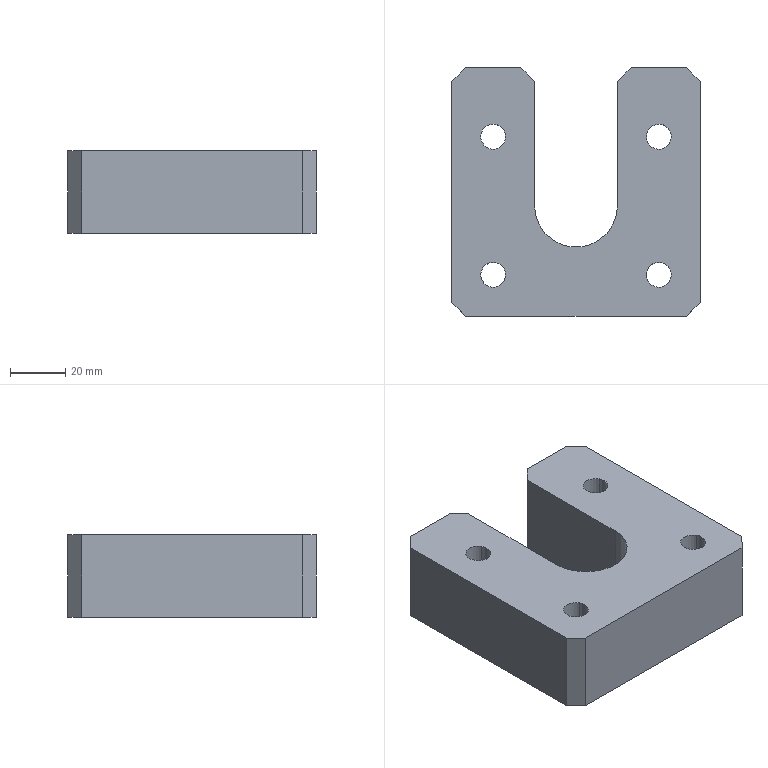Part | CATIA | 1 solid | 36 faces | box 90 x 90 x 30 mm | volume 170727 mm3 | plane 19 | cylinder 17 | commonest cylinder face diameters 9 x8 15 x8 30 x1
STEP:
#1=CARTESIAN_POINT('',(500.,-120.,-5.5));
#2=VERTEX_POINT('',#1);
#3=CARTESIAN_POINT('',(500.,-120.,24.5));
#4=VERTEX_POINT('',#3);
#5=CARTESIAN_POINT('',(500.,-120.,9.5));
#6=DIRECTION('',(0.,0.,-1.));
#7=VECTOR('',#6,1.);
#8=LINE('',#5,#7);
#9=EDGE_CURVE('',#2,#4,#8,.F.);
#10=ORIENTED_EDGE('',*,*,#9,.F.);
#11=CARTESIAN_POINT('',(495.,-125.,-5.5));
#12=VERTEX_POINT('',#11);
#13=CARTESIAN_POINT('',(497.5,-122.5,-5.5));
#14=DIRECTION('',(0.7071,0.7071,0.));
#15=VECTOR('',#14,1.);
#16=LINE('',#13,#15);
#17=EDGE_CURVE('',#2,#12,#16,.F.);
#18=ORIENTED_EDGE('',*,*,#17,.T.);
#19=CARTESIAN_POINT('',(495.,-125.,24.5));
#20=VERTEX_POINT('',#19);
#21=CARTESIAN_POINT('',(495.,-125.,9.5));
#22=DIRECTION('',(0.,0.,-1.));
#23=VECTOR('',#22,1.);
#24=LINE('',#21,#23);
#25=EDGE_CURVE('',#12,#20,#24,.F.);
#26=ORIENTED_EDGE('',*,*,#25,.T.);
#27=CARTESIAN_POINT('',(497.5,-122.5,24.5));
#28=DIRECTION('',(0.7071,0.7071,0.));
#29=VECTOR('',#28,1.);
#30=LINE('',#27,#29);
#31=EDGE_CURVE('',#20,#4,#30,.T.);
#32=ORIENTED_EDGE('',*,*,#31,.T.);
#33=EDGE_LOOP('',(#10,#18,#26,#32));
#34=FACE_OUTER_BOUND('',#33,.T.);
#35=CARTESIAN_POINT('',(495.,-125.,30.5));
#36=DIRECTION('',(0.7071,-0.7071,0.));
#37=DIRECTION('',(0.,0.,-1.));
#38=AXIS2_PLACEMENT_3D('',#35,#36,#37);
#39=PLANE('',#38);
#40=ADVANCED_FACE('',(#34),#39,.F.);
#41=CARTESIAN_POINT('',(495.,-205.,-5.5));
#42=VERTEX_POINT('',#41);
#43=CARTESIAN_POINT('',(495.,-205.,24.5));
#44=VERTEX_POINT('',#43);
#45=CARTESIAN_POINT('',(495.,-205.,9.5));
#46=DIRECTION('',(0.,0.,1.));
#47=VECTOR('',#46,1.);
#48=LINE('',#45,#47);
#49=EDGE_CURVE('',#42,#44,#48,.T.);
#50=ORIENTED_EDGE('',*,*,#49,.T.);
#51=CARTESIAN_POINT('',(495.,-165.,24.5));
#52=DIRECTION('',(0.,1.,0.));
#53=VECTOR('',#52,1.);
#54=LINE('',#51,#53);
#55=EDGE_CURVE('',#20,#44,#54,.F.);
#56=ORIENTED_EDGE('',*,*,#55,.F.);
#57=ORIENTED_EDGE('',*,*,#25,.F.);
#58=CARTESIAN_POINT('',(495.,-165.,-5.5));
#59=DIRECTION('',(0.,1.,0.));
#60=VECTOR('',#59,1.);
#61=LINE('',#58,#60);
#62=EDGE_CURVE('',#12,#42,#61,.F.);
#63=ORIENTED_EDGE('',*,*,#62,.T.);
#64=EDGE_LOOP('',(#50,#56,#57,#63));
#65=FACE_OUTER_BOUND('',#64,.T.);
#66=CARTESIAN_POINT('',(495.,-210.,-5.5));
#67=DIRECTION('',(1.,0.,0.));
#68=DIRECTION('',(0.,1.,0.));
#69=AXIS2_PLACEMENT_3D('',#66,#67,#68);
#70=PLANE('',#69);
#71=ADVANCED_FACE('',(#65),#70,.F.);
#72=ORIENTED_EDGE('',*,*,#49,.F.);
#73=CARTESIAN_POINT('',(500.,-210.,-5.5));
#74=VERTEX_POINT('',#73);
#75=CARTESIAN_POINT('',(497.5,-207.5,-5.5));
#76=DIRECTION('',(0.7071,-0.7071,0.));
#77=VECTOR('',#76,1.);
#78=LINE('',#75,#77);
#79=EDGE_CURVE('',#42,#74,#78,.T.);
#80=ORIENTED_EDGE('',*,*,#79,.T.);
#81=CARTESIAN_POINT('',(500.,-210.,24.5));
#82=VERTEX_POINT('',#81);
#83=CARTESIAN_POINT('',(500.,-210.,9.5));
#84=DIRECTION('',(0.,0.,1.));
#85=VECTOR('',#84,1.);
#86=LINE('',#83,#85);
#87=EDGE_CURVE('',#74,#82,#86,.T.);
#88=ORIENTED_EDGE('',*,*,#87,.T.);
#89=CARTESIAN_POINT('',(497.5,-207.5,24.5));
#90=DIRECTION('',(0.7071,-0.7071,0.));
#91=VECTOR('',#90,1.);
#92=LINE('',#89,#91);
#93=EDGE_CURVE('',#82,#44,#92,.F.);
#94=ORIENTED_EDGE('',*,*,#93,.T.);
#95=EDGE_LOOP('',(#72,#80,#88,#94));
#96=FACE_OUTER_BOUND('',#95,.T.);
#97=CARTESIAN_POINT('',(495.,-205.,-11.5));
#98=DIRECTION('',(0.7071,0.7071,0.));
#99=DIRECTION('',(0.,0.,1.));
#100=AXIS2_PLACEMENT_3D('',#97,#98,#99);
#101=PLANE('',#100);
#102=ADVANCED_FACE('',(#96),#101,.F.);
#103=CARTESIAN_POINT('',(580.,-210.,-5.5));
#104=VERTEX_POINT('',#103);
#105=CARTESIAN_POINT('',(580.,-210.,24.5));
#106=VERTEX_POINT('',#105);
#107=CARTESIAN_POINT('',(580.,-210.,9.5));
#108=DIRECTION('',(0.,0.,-1.));
#109=VECTOR('',#108,1.);
#110=LINE('',#107,#109);
#111=EDGE_CURVE('',#104,#106,#110,.F.);
#112=ORIENTED_EDGE('',*,*,#111,.T.);
#113=CARTESIAN_POINT('',(540.,-210.,24.5));
#114=DIRECTION('',(-1.,0.,0.));
#115=VECTOR('',#114,1.);
#116=LINE('',#113,#115);
#117=EDGE_CURVE('',#82,#106,#116,.F.);
#118=ORIENTED_EDGE('',*,*,#117,.F.);
#119=ORIENTED_EDGE('',*,*,#87,.F.);
#120=CARTESIAN_POINT('',(540.,-210.,-5.5));
#121=DIRECTION('',(-1.,0.,0.));
#122=VECTOR('',#121,1.);
#123=LINE('',#120,#122);
#124=EDGE_CURVE('',#74,#104,#123,.F.);
#125=ORIENTED_EDGE('',*,*,#124,.T.);
#126=EDGE_LOOP('',(#112,#118,#119,#125));
#127=FACE_OUTER_BOUND('',#126,.T.);
#128=CARTESIAN_POINT('',(585.,-210.,-5.5));
#129=DIRECTION('',(0.,1.,0.));
#130=DIRECTION('',(-1.,0.,0.));
#131=AXIS2_PLACEMENT_3D('',#128,#129,#130);
#132=PLANE('',#131);
#133=ADVANCED_FACE('',(#127),#132,.F.);
#134=ORIENTED_EDGE('',*,*,#111,.F.);
#135=CARTESIAN_POINT('',(585.,-205.,-5.5));
#136=VERTEX_POINT('',#135);
#137=CARTESIAN_POINT('',(582.5,-207.5,-5.5));
#138=DIRECTION('',(-0.7071,-0.7071,0.));
#139=VECTOR('',#138,1.);
#140=LINE('',#137,#139);
#141=EDGE_CURVE('',#104,#136,#140,.F.);
#142=ORIENTED_EDGE('',*,*,#141,.T.);
#143=CARTESIAN_POINT('',(585.,-205.,24.5));
#144=VERTEX_POINT('',#143);
#145=CARTESIAN_POINT('',(585.,-205.,9.5));
#146=DIRECTION('',(0.,0.,-1.));
#147=VECTOR('',#146,1.);
#148=LINE('',#145,#147);
#149=EDGE_CURVE('',#136,#144,#148,.F.);
#150=ORIENTED_EDGE('',*,*,#149,.T.);
#151=CARTESIAN_POINT('',(582.5,-207.5,24.5));
#152=DIRECTION('',(-0.7071,-0.7071,0.));
#153=VECTOR('',#152,1.);
#154=LINE('',#151,#153);
#155=EDGE_CURVE('',#144,#106,#154,.T.);
#156=ORIENTED_EDGE('',*,*,#155,.T.);
#157=EDGE_LOOP('',(#134,#142,#150,#156));
#158=FACE_OUTER_BOUND('',#157,.T.);
#159=CARTESIAN_POINT('',(585.,-205.,30.5));
#160=DIRECTION('',(-0.7071,0.7071,0.));
#161=DIRECTION('',(0.,0.,-1.));
#162=AXIS2_PLACEMENT_3D('',#159,#160,#161);
#163=PLANE('',#162);
#164=ADVANCED_FACE('',(#158),#163,.F.);
#165=CARTESIAN_POINT('',(585.,-125.,-5.5));
#166=VERTEX_POINT('',#165);
#167=CARTESIAN_POINT('',(585.,-125.,24.5));
#168=VERTEX_POINT('',#167);
#169=CARTESIAN_POINT('',(585.,-125.,9.5));
#170=DIRECTION('',(0.,0.,1.));
#171=VECTOR('',#170,1.);
#172=LINE('',#169,#171);
#173=EDGE_CURVE('',#166,#168,#172,.T.);
#174=ORIENTED_EDGE('',*,*,#173,.T.);
#175=CARTESIAN_POINT('',(585.,-165.,24.5));
#176=DIRECTION('',(0.,-1.,0.));
#177=VECTOR('',#176,1.);
#178=LINE('',#175,#177);
#179=EDGE_CURVE('',#144,#168,#178,.F.);
#180=ORIENTED_EDGE('',*,*,#179,.F.);
#181=ORIENTED_EDGE('',*,*,#149,.F.);
#182=CARTESIAN_POINT('',(585.,-165.,-5.5));
#183=DIRECTION('',(0.,-1.,0.));
#184=VECTOR('',#183,1.);
#185=LINE('',#182,#184);
#186=EDGE_CURVE('',#136,#166,#185,.F.);
#187=ORIENTED_EDGE('',*,*,#186,.T.);
#188=EDGE_LOOP('',(#174,#180,#181,#187));
#189=FACE_OUTER_BOUND('',#188,.T.);
#190=CARTESIAN_POINT('',(585.,-120.,-5.5));
#191=DIRECTION('',(-1.,0.,0.));
#192=DIRECTION('',(0.,-1.,0.));
#193=AXIS2_PLACEMENT_3D('',#190,#191,#192);
#194=PLANE('',#193);
#195=ADVANCED_FACE('',(#189),#194,.F.);
#196=ORIENTED_EDGE('',*,*,#173,.F.);
#197=CARTESIAN_POINT('',(580.,-120.,-5.5));
#198=VERTEX_POINT('',#197);
#199=CARTESIAN_POINT('',(582.5,-122.5,-5.5));
#200=DIRECTION('',(-0.7071,0.7071,0.));
#201=VECTOR('',#200,1.);
#202=LINE('',#199,#201);
#203=EDGE_CURVE('',#166,#198,#202,.T.);
#204=ORIENTED_EDGE('',*,*,#203,.T.);
#205=CARTESIAN_POINT('',(580.,-120.,24.5));
#206=VERTEX_POINT('',#205);
#207=CARTESIAN_POINT('',(580.,-120.,9.5));
#208=DIRECTION('',(0.,0.,1.));
#209=VECTOR('',#208,1.);
#210=LINE('',#207,#209);
#211=EDGE_CURVE('',#198,#206,#210,.T.);
#212=ORIENTED_EDGE('',*,*,#211,.T.);
#213=CARTESIAN_POINT('',(582.5,-122.5,24.5));
#214=DIRECTION('',(-0.7071,0.7071,0.));
#215=VECTOR('',#214,1.);
#216=LINE('',#213,#215);
#217=EDGE_CURVE('',#206,#168,#216,.F.);
#218=ORIENTED_EDGE('',*,*,#217,.T.);
#219=EDGE_LOOP('',(#196,#204,#212,#218));
#220=FACE_OUTER_BOUND('',#219,.T.);
#221=CARTESIAN_POINT('',(585.,-125.,-11.5));
#222=DIRECTION('',(-0.7071,-0.7071,0.));
#223=DIRECTION('',(0.,0.,1.));
#224=AXIS2_PLACEMENT_3D('',#221,#222,#223);
#225=PLANE('',#224);
#226=ADVANCED_FACE('',(#220),#225,.F.);
#227=CARTESIAN_POINT('',(576.582,-141.404,9.5));
#228=VERTEX_POINT('',#227);
#229=CARTESIAN_POINT('',(563.418,-148.596,9.5));
#230=VERTEX_POINT('',#229);
#231=CARTESIAN_POINT('',(570.,-145.,9.5));
#232=DIRECTION('',(0.,0.,1.));
#233=AXIS2_PLACEMENT_3D('',#231,#232,$);
#234=CIRCLE('',#233,7.5);
#235=EDGE_CURVE('',#228,#230,#234,.T.);
#236=ORIENTED_EDGE('',*,*,#235,.F.);
#237=CARTESIAN_POINT('',(570.,-145.,9.5));
#238=DIRECTION('',(0.,0.,1.));
#239=AXIS2_PLACEMENT_3D('',#237,#238,$);
#240=CIRCLE('',#239,7.5);
#241=EDGE_CURVE('',#230,#228,#240,.T.);
#242=ORIENTED_EDGE('',*,*,#241,.F.);
#243=EDGE_LOOP('',(#236,#242));
#244=FACE_OUTER_BOUND('',#243,.T.);
#245=CARTESIAN_POINT('',(566.051,-147.157,9.5));
#246=VERTEX_POINT('',#245);
#247=CARTESIAN_POINT('',(573.949,-142.843,9.5));
#248=VERTEX_POINT('',#247);
#249=CARTESIAN_POINT('',(570.,-145.,9.5));
#250=DIRECTION('',(0.,0.,1.));
#251=AXIS2_PLACEMENT_3D('',#249,#250,$);
#252=CIRCLE('',#251,4.5);
#253=EDGE_CURVE('',#246,#248,#252,.T.);
#254=ORIENTED_EDGE('',*,*,#253,.T.);
#255=CARTESIAN_POINT('',(570.,-145.,9.5));
#256=DIRECTION('',(0.,0.,1.));
#257=AXIS2_PLACEMENT_3D('',#255,#256,$);
#258=CIRCLE('',#257,4.5);
#259=EDGE_CURVE('',#248,#246,#258,.T.);
#260=ORIENTED_EDGE('',*,*,#259,.T.);
#261=EDGE_LOOP('',(#254,#260));
#262=FACE_BOUND('',#261,.T.);
#263=CARTESIAN_POINT('',(574.5,-195.,9.5));
#264=DIRECTION('',(0.,0.,1.));
#265=DIRECTION('',(1.,0.,0.));
#266=AXIS2_PLACEMENT_3D('',#263,#264,#265);
#267=PLANE('',#266);
#268=ADVANCED_FACE('',(#244,#262),#267,.F.);
#269=CARTESIAN_POINT('',(563.418,-148.596,-5.5));
#270=VERTEX_POINT('',#269);
#271=CARTESIAN_POINT('',(576.582,-141.404,-5.5));
#272=VERTEX_POINT('',#271);
#273=CARTESIAN_POINT('',(570.,-145.,-5.5));
#274=DIRECTION('',(0.,0.,1.));
#275=AXIS2_PLACEMENT_3D('',#273,#274,$);
#276=CIRCLE('',#275,7.5);
#277=EDGE_CURVE('',#270,#272,#276,.T.);
#278=ORIENTED_EDGE('',*,*,#277,.F.);
#279=CARTESIAN_POINT('',(563.418,-148.596,1.8));
#280=DIRECTION('',(0.,0.,1.));
#281=VECTOR('',#280,1.);
#282=LINE('',#279,#281);
#283=EDGE_CURVE('',#230,#270,#282,.F.);
#284=ORIENTED_EDGE('',*,*,#283,.F.);
#285=ORIENTED_EDGE('',*,*,#241,.T.);
#286=CARTESIAN_POINT('',(576.582,-141.404,1.8));
#287=DIRECTION('',(0.,0.,1.));
#288=VECTOR('',#287,1.);
#289=LINE('',#286,#288);
#290=EDGE_CURVE('',#228,#272,#289,.F.);
#291=ORIENTED_EDGE('',*,*,#290,.T.);
#292=EDGE_LOOP('',(#278,#284,#285,#291));
#293=FACE_OUTER_BOUND('',#292,.T.);
#294=CARTESIAN_POINT('',(570.,-145.,-5.4));
#295=DIRECTION('',(0.,0.,1.));
#296=DIRECTION('',(0.8776,0.4794,0.));
#297=AXIS2_PLACEMENT_3D('',#294,#295,#296);
#298=CYLINDRICAL_SURFACE('',#297,7.5);
#299=ADVANCED_FACE('',(#293),#298,.F.);
#300=CARTESIAN_POINT('',(570.,-145.,-5.5));
#301=DIRECTION('',(0.,0.,1.));
#302=AXIS2_PLACEMENT_3D('',#300,#301,$);
#303=CIRCLE('',#302,7.5);
#304=EDGE_CURVE('',#272,#270,#303,.T.);
#305=ORIENTED_EDGE('',*,*,#304,.F.);
#306=ORIENTED_EDGE('',*,*,#290,.F.);
#307=ORIENTED_EDGE('',*,*,#235,.T.);
#308=ORIENTED_EDGE('',*,*,#283,.T.);
#309=EDGE_LOOP('',(#305,#306,#307,#308));
#310=FACE_OUTER_BOUND('',#309,.T.);
#311=ADVANCED_FACE('',(#310),#298,.F.);
#312=CARTESIAN_POINT('',(573.949,-142.843,24.5));
#313=VERTEX_POINT('',#312);
#314=CARTESIAN_POINT('',(566.051,-147.157,24.5));
#315=VERTEX_POINT('',#314);
#316=CARTESIAN_POINT('',(570.,-145.,24.5));
#317=DIRECTION('',(0.,0.,1.));
#318=AXIS2_PLACEMENT_3D('',#316,#317,$);
#319=CIRCLE('',#318,4.5);
#320=EDGE_CURVE('',#313,#315,#319,.T.);
#321=ORIENTED_EDGE('',*,*,#320,.T.);
#322=CARTESIAN_POINT('',(566.051,-147.157,17.2));
#323=DIRECTION('',(0.,0.,1.));
#324=VECTOR('',#323,1.);
#325=LINE('',#322,#324);
#326=EDGE_CURVE('',#315,#246,#325,.F.);
#327=ORIENTED_EDGE('',*,*,#326,.T.);
#328=ORIENTED_EDGE('',*,*,#259,.F.);
#329=CARTESIAN_POINT('',(573.949,-142.843,17.2));
#330=DIRECTION('',(0.,0.,1.));
#331=VECTOR('',#330,1.);
#332=LINE('',#329,#331);
#333=EDGE_CURVE('',#313,#248,#332,.F.);
#334=ORIENTED_EDGE('',*,*,#333,.F.);
#335=EDGE_LOOP('',(#321,#327,#328,#334));
#336=FACE_OUTER_BOUND('',#335,.T.);
#337=CARTESIAN_POINT('',(570.,-145.,-5.4));
#338=DIRECTION('',(0.,0.,1.));
#339=DIRECTION('',(0.8776,0.4794,0.));
#340=AXIS2_PLACEMENT_3D('',#337,#338,#339);
#341=CYLINDRICAL_SURFACE('',#340,4.5);
#342=ADVANCED_FACE('',(#336),#341,.F.);
#343=CARTESIAN_POINT('',(570.,-145.,24.5));
#344=DIRECTION('',(0.,0.,1.));
#345=AXIS2_PLACEMENT_3D('',#343,#344,$);
#346=CIRCLE('',#345,4.5);
#347=EDGE_CURVE('',#315,#313,#346,.T.);
#348=ORIENTED_EDGE('',*,*,#347,.T.);
#349=ORIENTED_EDGE('',*,*,#333,.T.);
#350=ORIENTED_EDGE('',*,*,#253,.F.);
#351=ORIENTED_EDGE('',*,*,#326,.F.);
#352=EDGE_LOOP('',(#348,#349,#350,#351));
#353=FACE_OUTER_BOUND('',#352,.T.);
#354=ADVANCED_FACE('',(#353),#341,.F.);
#355=CARTESIAN_POINT('',(516.582,-191.404,9.5));
#356=VERTEX_POINT('',#355);
#357=CARTESIAN_POINT('',(503.418,-198.596,9.5));
#358=VERTEX_POINT('',#357);
#359=CARTESIAN_POINT('',(510.,-195.,9.5));
#360=DIRECTION('',(0.,0.,1.));
#361=AXIS2_PLACEMENT_3D('',#359,#360,$);
#362=CIRCLE('',#361,7.5);
#363=EDGE_CURVE('',#356,#358,#362,.T.);
#364=ORIENTED_EDGE('',*,*,#363,.F.);
#365=CARTESIAN_POINT('',(510.,-195.,9.5));
#366=DIRECTION('',(0.,0.,1.));
#367=AXIS2_PLACEMENT_3D('',#365,#366,$);
#368=CIRCLE('',#367,7.5);
#369=EDGE_CURVE('',#358,#356,#368,.T.);
#370=ORIENTED_EDGE('',*,*,#369,.F.);
#371=EDGE_LOOP('',(#364,#370));
#372=FACE_OUTER_BOUND('',#371,.T.);
#373=CARTESIAN_POINT('',(506.051,-197.157,9.5));
#374=VERTEX_POINT('',#373);
#375=CARTESIAN_POINT('',(513.949,-192.843,9.5));
#376=VERTEX_POINT('',#375);
#377=CARTESIAN_POINT('',(510.,-195.,9.5));
#378=DIRECTION('',(0.,0.,1.));
#379=AXIS2_PLACEMENT_3D('',#377,#378,$);
#380=CIRCLE('',#379,4.5);
#381=EDGE_CURVE('',#374,#376,#380,.T.);
#382=ORIENTED_EDGE('',*,*,#381,.T.);
#383=CARTESIAN_POINT('',(510.,-195.,9.5));
#384=DIRECTION('',(0.,0.,1.));
#385=AXIS2_PLACEMENT_3D('',#383,#384,$);
#386=CIRCLE('',#385,4.5);
#387=EDGE_CURVE('',#376,#374,#386,.T.);
#388=ORIENTED_EDGE('',*,*,#387,.T.);
#389=EDGE_LOOP('',(#382,#388));
#390=FACE_BOUND('',#389,.T.);
#391=ADVANCED_FACE('',(#372,#390),#267,.F.);
#392=CARTESIAN_POINT('',(503.418,-198.596,-5.5));
#393=VERTEX_POINT('',#392);
#394=CARTESIAN_POINT('',(516.582,-191.404,-5.5));
#395=VERTEX_POINT('',#394);
#396=CARTESIAN_POINT('',(510.,-195.,-5.5));
#397=DIRECTION('',(0.,0.,1.));
#398=AXIS2_PLACEMENT_3D('',#396,#397,$);
#399=CIRCLE('',#398,7.5);
#400=EDGE_CURVE('',#393,#395,#399,.T.);
#401=ORIENTED_EDGE('',*,*,#400,.F.);
#402=CARTESIAN_POINT('',(503.418,-198.596,1.8));
#403=DIRECTION('',(0.,0.,1.));
#404=VECTOR('',#403,1.);
#405=LINE('',#402,#404);
#406=EDGE_CURVE('',#358,#393,#405,.F.);
#407=ORIENTED_EDGE('',*,*,#406,.F.);
#408=ORIENTED_EDGE('',*,*,#369,.T.);
#409=CARTESIAN_POINT('',(516.582,-191.404,1.8));
#410=DIRECTION('',(0.,0.,1.));
#411=VECTOR('',#410,1.);
#412=LINE('',#409,#411);
#413=EDGE_CURVE('',#356,#395,#412,.F.);
#414=ORIENTED_EDGE('',*,*,#413,.T.);
#415=EDGE_LOOP('',(#401,#407,#408,#414));
#416=FACE_OUTER_BOUND('',#415,.T.);
#417=CARTESIAN_POINT('',(510.,-195.,-5.4));
#418=DIRECTION('',(0.,0.,1.));
#419=DIRECTION('',(0.8776,0.4794,0.));
#420=AXIS2_PLACEMENT_3D('',#417,#418,#419);
#421=CYLINDRICAL_SURFACE('',#420,7.5);
#422=ADVANCED_FACE('',(#416),#421,.F.);
#423=CARTESIAN_POINT('',(510.,-195.,-5.5));
#424=DIRECTION('',(0.,0.,1.));
#425=AXIS2_PLACEMENT_3D('',#423,#424,$);
#426=CIRCLE('',#425,7.5);
#427=EDGE_CURVE('',#395,#393,#426,.T.);
#428=ORIENTED_EDGE('',*,*,#427,.F.);
#429=ORIENTED_EDGE('',*,*,#413,.F.);
#430=ORIENTED_EDGE('',*,*,#363,.T.);
#431=ORIENTED_EDGE('',*,*,#406,.T.);
#432=EDGE_LOOP('',(#428,#429,#430,#431));
#433=FACE_OUTER_BOUND('',#432,.T.);
#434=ADVANCED_FACE('',(#433),#421,.F.);
#435=CARTESIAN_POINT('',(513.949,-192.843,24.5));
#436=VERTEX_POINT('',#435);
#437=CARTESIAN_POINT('',(506.051,-197.157,24.5));
#438=VERTEX_POINT('',#437);
#439=CARTESIAN_POINT('',(510.,-195.,24.5));
#440=DIRECTION('',(0.,0.,1.));
#441=AXIS2_PLACEMENT_3D('',#439,#440,$);
#442=CIRCLE('',#441,4.5);
#443=EDGE_CURVE('',#436,#438,#442,.T.);
#444=ORIENTED_EDGE('',*,*,#443,.T.);
#445=CARTESIAN_POINT('',(506.051,-197.157,17.2));
#446=DIRECTION('',(0.,0.,1.));
#447=VECTOR('',#446,1.);
#448=LINE('',#445,#447);
#449=EDGE_CURVE('',#438,#374,#448,.F.);
#450=ORIENTED_EDGE('',*,*,#449,.T.);
#451=ORIENTED_EDGE('',*,*,#387,.F.);
#452=CARTESIAN_POINT('',(513.949,-192.843,17.2));
#453=DIRECTION('',(0.,0.,1.));
#454=VECTOR('',#453,1.);
#455=LINE('',#452,#454);
#456=EDGE_CURVE('',#436,#376,#455,.F.);
#457=ORIENTED_EDGE('',*,*,#456,.F.);
#458=EDGE_LOOP('',(#444,#450,#451,#457));
#459=FACE_OUTER_BOUND('',#458,.T.);
#460=CARTESIAN_POINT('',(510.,-195.,-5.4));
#461=DIRECTION('',(0.,0.,1.));
#462=DIRECTION('',(0.8776,0.4794,0.));
#463=AXIS2_PLACEMENT_3D('',#460,#461,#462);
#464=CYLINDRICAL_SURFACE('',#463,4.5);
#465=ADVANCED_FACE('',(#459),#464,.F.);
#466=CARTESIAN_POINT('',(510.,-195.,24.5));
#467=DIRECTION('',(0.,0.,1.));
#468=AXIS2_PLACEMENT_3D('',#466,#467,$);
#469=CIRCLE('',#468,4.5);
#470=EDGE_CURVE('',#438,#436,#469,.T.);
#471=ORIENTED_EDGE('',*,*,#470,.T.);
#472=ORIENTED_EDGE('',*,*,#456,.T.);
#473=ORIENTED_EDGE('',*,*,#381,.F.);
#474=ORIENTED_EDGE('',*,*,#449,.F.);
#475=EDGE_LOOP('',(#471,#472,#473,#474));
#476=FACE_OUTER_BOUND('',#475,.T.);
#477=ADVANCED_FACE('',(#476),#464,.F.);
#478=CARTESIAN_POINT('',(516.582,-141.404,9.5));
#479=VERTEX_POINT('',#478);
#480=CARTESIAN_POINT('',(503.418,-148.596,9.5));
#481=VERTEX_POINT('',#480);
#482=CARTESIAN_POINT('',(510.,-145.,9.5));
#483=DIRECTION('',(0.,0.,1.));
#484=AXIS2_PLACEMENT_3D('',#482,#483,$);
#485=CIRCLE('',#484,7.5);
#486=EDGE_CURVE('',#479,#481,#485,.T.);
#487=ORIENTED_EDGE('',*,*,#486,.F.);
#488=CARTESIAN_POINT('',(510.,-145.,9.5));
#489=DIRECTION('',(0.,0.,1.));
#490=AXIS2_PLACEMENT_3D('',#488,#489,$);
#491=CIRCLE('',#490,7.5);
#492=EDGE_CURVE('',#481,#479,#491,.T.);
#493=ORIENTED_EDGE('',*,*,#492,.F.);
#494=EDGE_LOOP('',(#487,#493));
#495=FACE_OUTER_BOUND('',#494,.T.);
#496=CARTESIAN_POINT('',(506.051,-147.157,9.5));
#497=VERTEX_POINT('',#496);
#498=CARTESIAN_POINT('',(513.949,-142.843,9.5));
#499=VERTEX_POINT('',#498);
#500=CARTESIAN_POINT('',(510.,-145.,9.5));
#501=DIRECTION('',(0.,0.,1.));
#502=AXIS2_PLACEMENT_3D('',#500,#501,$);
#503=CIRCLE('',#502,4.5);
#504=EDGE_CURVE('',#497,#499,#503,.T.);
#505=ORIENTED_EDGE('',*,*,#504,.T.);
#506=CARTESIAN_POINT('',(510.,-145.,9.5));
#507=DIRECTION('',(0.,0.,1.));
#508=AXIS2_PLACEMENT_3D('',#506,#507,$);
#509=CIRCLE('',#508,4.5);
#510=EDGE_CURVE('',#499,#497,#509,.T.);
#511=ORIENTED_EDGE('',*,*,#510,.T.);
#512=EDGE_LOOP('',(#505,#511));
#513=FACE_BOUND('',#512,.T.);
#514=ADVANCED_FACE('',(#495,#513),#267,.F.);
#515=CARTESIAN_POINT('',(503.418,-148.596,-5.5));
#516=VERTEX_POINT('',#515);
#517=CARTESIAN_POINT('',(516.582,-141.404,-5.5));
#518=VERTEX_POINT('',#517);
#519=CARTESIAN_POINT('',(510.,-145.,-5.5));
#520=DIRECTION('',(0.,0.,1.));
#521=AXIS2_PLACEMENT_3D('',#519,#520,$);
#522=CIRCLE('',#521,7.5);
#523=EDGE_CURVE('',#516,#518,#522,.T.);
#524=ORIENTED_EDGE('',*,*,#523,.F.);
#525=CARTESIAN_POINT('',(503.418,-148.596,1.8));
#526=DIRECTION('',(0.,0.,1.));
#527=VECTOR('',#526,1.);
#528=LINE('',#525,#527);
#529=EDGE_CURVE('',#481,#516,#528,.F.);
#530=ORIENTED_EDGE('',*,*,#529,.F.);
#531=ORIENTED_EDGE('',*,*,#492,.T.);
#532=CARTESIAN_POINT('',(516.582,-141.404,1.8));
#533=DIRECTION('',(0.,0.,1.));
#534=VECTOR('',#533,1.);
#535=LINE('',#532,#534);
#536=EDGE_CURVE('',#479,#518,#535,.F.);
#537=ORIENTED_EDGE('',*,*,#536,.T.);
#538=EDGE_LOOP('',(#524,#530,#531,#537));
#539=FACE_OUTER_BOUND('',#538,.T.);
#540=CARTESIAN_POINT('',(510.,-145.,-5.4));
#541=DIRECTION('',(0.,0.,1.));
#542=DIRECTION('',(0.8776,0.4794,0.));
#543=AXIS2_PLACEMENT_3D('',#540,#541,#542);
#544=CYLINDRICAL_SURFACE('',#543,7.5);
#545=ADVANCED_FACE('',(#539),#544,.F.);
#546=CARTESIAN_POINT('',(510.,-145.,-5.5));
#547=DIRECTION('',(0.,0.,1.));
#548=AXIS2_PLACEMENT_3D('',#546,#547,$);
#549=CIRCLE('',#548,7.5);
#550=EDGE_CURVE('',#518,#516,#549,.T.);
#551=ORIENTED_EDGE('',*,*,#550,.F.);
#552=ORIENTED_EDGE('',*,*,#536,.F.);
#553=ORIENTED_EDGE('',*,*,#486,.T.);
#554=ORIENTED_EDGE('',*,*,#529,.T.);
#555=EDGE_LOOP('',(#551,#552,#553,#554));
#556=FACE_OUTER_BOUND('',#555,.T.);
#557=ADVANCED_FACE('',(#556),#544,.F.);
#558=CARTESIAN_POINT('',(513.949,-142.843,24.5));
#559=VERTEX_POINT('',#558);
#560=CARTESIAN_POINT('',(506.051,-147.157,24.5));
#561=VERTEX_POINT('',#560);
#562=CARTESIAN_POINT('',(510.,-145.,24.5));
#563=DIRECTION('',(0.,0.,1.));
#564=AXIS2_PLACEMENT_3D('',#562,#563,$);
#565=CIRCLE('',#564,4.5);
#566=EDGE_CURVE('',#559,#561,#565,.T.);
#567=ORIENTED_EDGE('',*,*,#566,.T.);
#568=CARTESIAN_POINT('',(506.051,-147.157,17.2));
#569=DIRECTION('',(0.,0.,1.));
#570=VECTOR('',#569,1.);
#571=LINE('',#568,#570);
#572=EDGE_CURVE('',#561,#497,#571,.F.);
#573=ORIENTED_EDGE('',*,*,#572,.T.);
#574=ORIENTED_EDGE('',*,*,#510,.F.);
#575=CARTESIAN_POINT('',(513.949,-142.843,17.2));
#576=DIRECTION('',(0.,0.,1.));
#577=VECTOR('',#576,1.);
#578=LINE('',#575,#577);
#579=EDGE_CURVE('',#559,#499,#578,.F.);
#580=ORIENTED_EDGE('',*,*,#579,.F.);
#581=EDGE_LOOP('',(#567,#573,#574,#580));
#582=FACE_OUTER_BOUND('',#581,.T.);
#583=CARTESIAN_POINT('',(510.,-145.,-5.4));
#584=DIRECTION('',(0.,0.,1.));
#585=DIRECTION('',(0.8776,0.4794,0.));
#586=AXIS2_PLACEMENT_3D('',#583,#584,#585);
#587=CYLINDRICAL_SURFACE('',#586,4.5);
#588=ADVANCED_FACE('',(#582),#587,.F.);
#589=CARTESIAN_POINT('',(510.,-145.,24.5));
#590=DIRECTION('',(0.,0.,1.));
#591=AXIS2_PLACEMENT_3D('',#589,#590,$);
#592=CIRCLE('',#591,4.5);
#593=EDGE_CURVE('',#561,#559,#592,.T.);
#594=ORIENTED_EDGE('',*,*,#593,.T.);
#595=ORIENTED_EDGE('',*,*,#579,.T.);
#596=ORIENTED_EDGE('',*,*,#504,.F.);
#597=ORIENTED_EDGE('',*,*,#572,.F.);
#598=EDGE_LOOP('',(#594,#595,#596,#597));
#599=FACE_OUTER_BOUND('',#598,.T.);
#600=ADVANCED_FACE('',(#599),#587,.F.);
#601=CARTESIAN_POINT('',(576.582,-191.404,9.5));
#602=VERTEX_POINT('',#601);
#603=CARTESIAN_POINT('',(563.418,-198.596,9.5));
#604=VERTEX_POINT('',#603);
#605=CARTESIAN_POINT('',(570.,-195.,9.5));
#606=DIRECTION('',(0.,0.,1.));
#607=AXIS2_PLACEMENT_3D('',#605,#606,$);
#608=CIRCLE('',#607,7.5);
#609=EDGE_CURVE('',#602,#604,#608,.T.);
#610=ORIENTED_EDGE('',*,*,#609,.F.);
#611=CARTESIAN_POINT('',(570.,-195.,9.5));
#612=DIRECTION('',(0.,0.,1.));
#613=AXIS2_PLACEMENT_3D('',#611,#612,$);
#614=CIRCLE('',#613,7.5);
#615=EDGE_CURVE('',#604,#602,#614,.T.);
#616=ORIENTED_EDGE('',*,*,#615,.F.);
#617=EDGE_LOOP('',(#610,#616));
#618=FACE_OUTER_BOUND('',#617,.T.);
#619=CARTESIAN_POINT('',(566.051,-197.157,9.5));
#620=VERTEX_POINT('',#619);
#621=CARTESIAN_POINT('',(573.949,-192.843,9.5));
#622=VERTEX_POINT('',#621);
#623=CARTESIAN_POINT('',(570.,-195.,9.5));
#624=DIRECTION('',(0.,0.,1.));
#625=AXIS2_PLACEMENT_3D('',#623,#624,$);
#626=CIRCLE('',#625,4.5);
#627=EDGE_CURVE('',#620,#622,#626,.T.);
#628=ORIENTED_EDGE('',*,*,#627,.T.);
#629=CARTESIAN_POINT('',(570.,-195.,9.5));
#630=DIRECTION('',(0.,0.,1.));
#631=AXIS2_PLACEMENT_3D('',#629,#630,$);
#632=CIRCLE('',#631,4.5);
#633=EDGE_CURVE('',#622,#620,#632,.T.);
#634=ORIENTED_EDGE('',*,*,#633,.T.);
#635=EDGE_LOOP('',(#628,#634));
#636=FACE_BOUND('',#635,.T.);
#637=ADVANCED_FACE('',(#618,#636),#267,.F.);
#638=CARTESIAN_POINT('',(563.418,-198.596,-5.5));
#639=VERTEX_POINT('',#638);
#640=CARTESIAN_POINT('',(576.582,-191.404,-5.5));
#641=VERTEX_POINT('',#640);
#642=CARTESIAN_POINT('',(570.,-195.,-5.5));
#643=DIRECTION('',(0.,0.,1.));
#644=AXIS2_PLACEMENT_3D('',#642,#643,$);
#645=CIRCLE('',#644,7.5);
#646=EDGE_CURVE('',#639,#641,#645,.T.);
#647=ORIENTED_EDGE('',*,*,#646,.F.);
#648=CARTESIAN_POINT('',(563.418,-198.596,1.8));
#649=DIRECTION('',(0.,0.,1.));
#650=VECTOR('',#649,1.);
#651=LINE('',#648,#650);
#652=EDGE_CURVE('',#604,#639,#651,.F.);
#653=ORIENTED_EDGE('',*,*,#652,.F.);
#654=ORIENTED_EDGE('',*,*,#615,.T.);
#655=CARTESIAN_POINT('',(576.582,-191.404,1.8));
#656=DIRECTION('',(0.,0.,1.));
#657=VECTOR('',#656,1.);
#658=LINE('',#655,#657);
#659=EDGE_CURVE('',#602,#641,#658,.F.);
#660=ORIENTED_EDGE('',*,*,#659,.T.);
#661=EDGE_LOOP('',(#647,#653,#654,#660));
#662=FACE_OUTER_BOUND('',#661,.T.);
#663=CARTESIAN_POINT('',(570.,-195.,-5.4));
#664=DIRECTION('',(0.,0.,1.));
#665=DIRECTION('',(0.8776,0.4794,0.));
#666=AXIS2_PLACEMENT_3D('',#663,#664,#665);
#667=CYLINDRICAL_SURFACE('',#666,7.5);
#668=ADVANCED_FACE('',(#662),#667,.F.);
#669=CARTESIAN_POINT('',(570.,-195.,-5.5));
#670=DIRECTION('',(0.,0.,1.));
#671=AXIS2_PLACEMENT_3D('',#669,#670,$);
#672=CIRCLE('',#671,7.5);
#673=EDGE_CURVE('',#641,#639,#672,.T.);
#674=ORIENTED_EDGE('',*,*,#673,.F.);
#675=ORIENTED_EDGE('',*,*,#659,.F.);
#676=ORIENTED_EDGE('',*,*,#609,.T.);
#677=ORIENTED_EDGE('',*,*,#652,.T.);
#678=EDGE_LOOP('',(#674,#675,#676,#677));
#679=FACE_OUTER_BOUND('',#678,.T.);
#680=ADVANCED_FACE('',(#679),#667,.F.);
#681=CARTESIAN_POINT('',(573.949,-192.843,24.5));
#682=VERTEX_POINT('',#681);
#683=CARTESIAN_POINT('',(566.051,-197.157,24.5));
#684=VERTEX_POINT('',#683);
#685=CARTESIAN_POINT('',(570.,-195.,24.5));
#686=DIRECTION('',(0.,0.,1.));
#687=AXIS2_PLACEMENT_3D('',#685,#686,$);
#688=CIRCLE('',#687,4.5);
#689=EDGE_CURVE('',#682,#684,#688,.T.);
#690=ORIENTED_EDGE('',*,*,#689,.T.);
#691=CARTESIAN_POINT('',(566.051,-197.157,17.2));
#692=DIRECTION('',(0.,0.,1.));
#693=VECTOR('',#692,1.);
#694=LINE('',#691,#693);
#695=EDGE_CURVE('',#684,#620,#694,.F.);
#696=ORIENTED_EDGE('',*,*,#695,.T.);
#697=ORIENTED_EDGE('',*,*,#633,.F.);
#698=CARTESIAN_POINT('',(573.949,-192.843,17.2));
#699=DIRECTION('',(0.,0.,1.));
#700=VECTOR('',#699,1.);
#701=LINE('',#698,#700);
#702=EDGE_CURVE('',#682,#622,#701,.F.);
#703=ORIENTED_EDGE('',*,*,#702,.F.);
#704=EDGE_LOOP('',(#690,#696,#697,#703));
#705=FACE_OUTER_BOUND('',#704,.T.);
#706=CARTESIAN_POINT('',(570.,-195.,-5.4));
#707=DIRECTION('',(0.,0.,1.));
#708=DIRECTION('',(0.8776,0.4794,0.));
#709=AXIS2_PLACEMENT_3D('',#706,#707,#708);
#710=CYLINDRICAL_SURFACE('',#709,4.5);
#711=ADVANCED_FACE('',(#705),#710,.F.);
#712=CARTESIAN_POINT('',(570.,-195.,24.5));
#713=DIRECTION('',(0.,0.,1.));
#714=AXIS2_PLACEMENT_3D('',#712,#713,$);
#715=CIRCLE('',#714,4.5);
#716=EDGE_CURVE('',#684,#682,#715,.T.);
#717=ORIENTED_EDGE('',*,*,#716,.T.);
#718=ORIENTED_EDGE('',*,*,#702,.T.);
#719=ORIENTED_EDGE('',*,*,#627,.F.);
#720=ORIENTED_EDGE('',*,*,#695,.F.);
#721=EDGE_LOOP('',(#717,#718,#719,#720));
#722=FACE_OUTER_BOUND('',#721,.T.);
#723=ADVANCED_FACE('',(#722),#710,.F.);
#724=CARTESIAN_POINT('',(555.,-170.,-5.5));
#725=VERTEX_POINT('',#724);
#726=CARTESIAN_POINT('',(555.,-170.,24.5));
#727=VERTEX_POINT('',#726);
#728=CARTESIAN_POINT('',(555.,-170.,9.5));
#729=DIRECTION('',(0.,0.,-1.));
#730=VECTOR('',#729,1.);
#731=LINE('',#728,#730);
#732=EDGE_CURVE('',#725,#727,#731,.F.);
#733=ORIENTED_EDGE('',*,*,#732,.F.);
#734=CARTESIAN_POINT('',(525.,-170.,-5.5));
#735=VERTEX_POINT('',#734);
#736=CARTESIAN_POINT('',(540.,-170.,-5.5));
#737=DIRECTION('',(0.,0.,-1.));
#738=AXIS2_PLACEMENT_3D('',#736,#737,$);
#739=CIRCLE('',#738,15.);
#740=EDGE_CURVE('',#725,#735,#739,.T.);
#741=ORIENTED_EDGE('',*,*,#740,.T.);
#742=CARTESIAN_POINT('',(525.,-170.,24.5));
#743=VERTEX_POINT('',#742);
#744=CARTESIAN_POINT('',(525.,-170.,9.5));
#745=DIRECTION('',(0.,0.,-1.));
#746=VECTOR('',#745,1.);
#747=LINE('',#744,#746);
#748=EDGE_CURVE('',#735,#743,#747,.F.);
#749=ORIENTED_EDGE('',*,*,#748,.T.);
#750=CARTESIAN_POINT('',(540.,-170.,24.5));
#751=DIRECTION('',(0.,0.,-1.));
#752=AXIS2_PLACEMENT_3D('',#750,#751,$);
#753=CIRCLE('',#752,15.);
#754=EDGE_CURVE('',#727,#743,#753,.T.);
#755=ORIENTED_EDGE('',*,*,#754,.F.);
#756=EDGE_LOOP('',(#733,#741,#749,#755));
#757=FACE_OUTER_BOUND('',#756,.T.);
#758=CARTESIAN_POINT('',(540.,-170.,9.5));
#759=DIRECTION('',(0.,0.,-1.));
#760=DIRECTION('',(1.,0.,0.));
#761=AXIS2_PLACEMENT_3D('',#758,#759,#760);
#762=CYLINDRICAL_SURFACE('',#761,15.);
#763=ADVANCED_FACE('',(#757),#762,.F.);
#764=CARTESIAN_POINT('',(560.,-120.,24.5));
#765=VERTEX_POINT('',#764);
#766=CARTESIAN_POINT('',(560.,-120.,-5.5));
#767=VERTEX_POINT('',#766);
#768=CARTESIAN_POINT('',(560.,-120.,9.5));
#769=DIRECTION('',(0.,0.,1.));
#770=VECTOR('',#769,1.);
#771=LINE('',#768,#770);
#772=EDGE_CURVE('',#765,#767,#771,.F.);
#773=ORIENTED_EDGE('',*,*,#772,.F.);
#774=CARTESIAN_POINT('',(570.,-120.,24.5));
#775=DIRECTION('',(1.,0.,0.));
#776=VECTOR('',#775,1.);
#777=LINE('',#774,#776);
#778=EDGE_CURVE('',#206,#765,#777,.F.);
#779=ORIENTED_EDGE('',*,*,#778,.F.);
#780=ORIENTED_EDGE('',*,*,#211,.F.);
#781=CARTESIAN_POINT('',(570.,-120.,-5.5));
#782=DIRECTION('',(1.,0.,0.));
#783=VECTOR('',#782,1.);
#784=LINE('',#781,#783);
#785=EDGE_CURVE('',#198,#767,#784,.F.);
#786=ORIENTED_EDGE('',*,*,#785,.T.);
#787=EDGE_LOOP('',(#773,#779,#780,#786));
#788=FACE_OUTER_BOUND('',#787,.T.);
#789=CARTESIAN_POINT('',(495.,-120.,-5.5));
#790=DIRECTION('',(0.,-1.,0.));
#791=DIRECTION('',(1.,0.,0.));
#792=AXIS2_PLACEMENT_3D('',#789,#790,#791);
#793=PLANE('',#792);
#794=ADVANCED_FACE('',(#788),#793,.F.);
#795=CARTESIAN_POINT('',(555.,-125.,24.5));
#796=VERTEX_POINT('',#795);
#797=CARTESIAN_POINT('',(555.,-125.,-5.5));
#798=VERTEX_POINT('',#797);
#799=CARTESIAN_POINT('',(555.,-125.,9.5));
#800=DIRECTION('',(0.,0.,1.));
#801=VECTOR('',#800,1.);
#802=LINE('',#799,#801);
#803=EDGE_CURVE('',#796,#798,#802,.F.);
#804=ORIENTED_EDGE('',*,*,#803,.T.);
#805=CARTESIAN_POINT('',(555.,-147.5,-5.5));
#806=DIRECTION('',(0.,1.,0.));
#807=VECTOR('',#806,1.);
#808=LINE('',#805,#807);
#809=EDGE_CURVE('',#798,#725,#808,.F.);
#810=ORIENTED_EDGE('',*,*,#809,.T.);
#811=ORIENTED_EDGE('',*,*,#732,.T.);
#812=CARTESIAN_POINT('',(555.,-147.5,24.5));
#813=DIRECTION('',(0.,1.,0.));
#814=VECTOR('',#813,1.);
#815=LINE('',#812,#814);
#816=EDGE_CURVE('',#796,#727,#815,.F.);
#817=ORIENTED_EDGE('',*,*,#816,.F.);
#818=EDGE_LOOP('',(#804,#810,#811,#817));
#819=FACE_OUTER_BOUND('',#818,.T.);
#820=CARTESIAN_POINT('',(555.,-170.,-5.5));
#821=DIRECTION('',(1.,0.,0.));
#822=DIRECTION('',(0.,1.,0.));
#823=AXIS2_PLACEMENT_3D('',#820,#821,#822);
#824=PLANE('',#823);
#825=ADVANCED_FACE('',(#819),#824,.F.);
#826=ORIENTED_EDGE('',*,*,#803,.F.);
#827=CARTESIAN_POINT('',(557.5,-122.5,24.5));
#828=DIRECTION('',(-0.7071,-0.7071,0.));
#829=VECTOR('',#828,1.);
#830=LINE('',#827,#829);
#831=EDGE_CURVE('',#796,#765,#830,.F.);
#832=ORIENTED_EDGE('',*,*,#831,.T.);
#833=ORIENTED_EDGE('',*,*,#772,.T.);
#834=CARTESIAN_POINT('',(557.5,-122.5,-5.5));
#835=DIRECTION('',(-0.7071,-0.7071,0.));
#836=VECTOR('',#835,1.);
#837=LINE('',#834,#836);
#838=EDGE_CURVE('',#767,#798,#837,.T.);
#839=ORIENTED_EDGE('',*,*,#838,.T.);
#840=EDGE_LOOP('',(#826,#832,#833,#839));
#841=FACE_OUTER_BOUND('',#840,.T.);
#842=CARTESIAN_POINT('',(560.,-120.,-11.5));
#843=DIRECTION('',(0.7071,-0.7071,0.));
#844=DIRECTION('',(0.,0.,1.));
#845=AXIS2_PLACEMENT_3D('',#842,#843,#844);
#846=PLANE('',#845);
#847=ADVANCED_FACE('',(#841),#846,.F.);
#848=CARTESIAN_POINT('',(520.,-120.,24.5));
#849=VERTEX_POINT('',#848);
#850=CARTESIAN_POINT('',(520.,-120.,-5.5));
#851=VERTEX_POINT('',#850);
#852=CARTESIAN_POINT('',(520.,-120.,9.5));
#853=DIRECTION('',(0.,0.,1.));
#854=VECTOR('',#853,1.);
#855=LINE('',#852,#854);
#856=EDGE_CURVE('',#849,#851,#855,.F.);
#857=ORIENTED_EDGE('',*,*,#856,.T.);
#858=CARTESIAN_POINT('',(510.,-120.,-5.5));
#859=DIRECTION('',(1.,0.,0.));
#860=VECTOR('',#859,1.);
#861=LINE('',#858,#860);
#862=EDGE_CURVE('',#851,#2,#861,.F.);
#863=ORIENTED_EDGE('',*,*,#862,.T.);
#864=ORIENTED_EDGE('',*,*,#9,.T.);
#865=CARTESIAN_POINT('',(510.,-120.,24.5));
#866=DIRECTION('',(1.,0.,0.));
#867=VECTOR('',#866,1.);
#868=LINE('',#865,#867);
#869=EDGE_CURVE('',#849,#4,#868,.F.);
#870=ORIENTED_EDGE('',*,*,#869,.F.);
#871=EDGE_LOOP('',(#857,#863,#864,#870));
#872=FACE_OUTER_BOUND('',#871,.T.);
#873=ADVANCED_FACE('',(#872),#793,.F.);
#874=CARTESIAN_POINT('',(525.,-125.,24.5));
#875=VERTEX_POINT('',#874);
#876=CARTESIAN_POINT('',(525.,-125.,-5.5));
#877=VERTEX_POINT('',#876);
#878=CARTESIAN_POINT('',(525.,-125.,9.5));
#879=DIRECTION('',(0.,0.,1.));
#880=VECTOR('',#879,1.);
#881=LINE('',#878,#880);
#882=EDGE_CURVE('',#875,#877,#881,.F.);
#883=ORIENTED_EDGE('',*,*,#882,.F.);
#884=CARTESIAN_POINT('',(525.,-147.5,24.5));
#885=DIRECTION('',(0.,-1.,0.));
#886=VECTOR('',#885,1.);
#887=LINE('',#884,#886);
#888=EDGE_CURVE('',#743,#875,#887,.F.);
#889=ORIENTED_EDGE('',*,*,#888,.F.);
#890=ORIENTED_EDGE('',*,*,#748,.F.);
#891=CARTESIAN_POINT('',(525.,-147.5,-5.5));
#892=DIRECTION('',(0.,-1.,0.));
#893=VECTOR('',#892,1.);
#894=LINE('',#891,#893);
#895=EDGE_CURVE('',#735,#877,#894,.F.);
#896=ORIENTED_EDGE('',*,*,#895,.T.);
#897=EDGE_LOOP('',(#883,#889,#890,#896));
#898=FACE_OUTER_BOUND('',#897,.T.);
#899=CARTESIAN_POINT('',(525.,-110.,-5.5));
#900=DIRECTION('',(-1.,0.,0.));
#901=DIRECTION('',(0.,-1.,0.));
#902=AXIS2_PLACEMENT_3D('',#899,#900,#901);
#903=PLANE('',#902);
#904=ADVANCED_FACE('',(#898),#903,.F.);
#905=CARTESIAN_POINT('',(522.5,-122.5,-5.5));
#906=DIRECTION('',(0.7071,-0.7071,0.));
#907=VECTOR('',#906,1.);
#908=LINE('',#905,#907);
#909=EDGE_CURVE('',#877,#851,#908,.F.);
#910=ORIENTED_EDGE('',*,*,#909,.F.);
#911=ORIENTED_EDGE('',*,*,#895,.F.);
#912=ORIENTED_EDGE('',*,*,#740,.F.);
#913=ORIENTED_EDGE('',*,*,#809,.F.);
#914=ORIENTED_EDGE('',*,*,#838,.F.);
#915=ORIENTED_EDGE('',*,*,#785,.F.);
#916=ORIENTED_EDGE('',*,*,#203,.F.);
#917=ORIENTED_EDGE('',*,*,#186,.F.);
#918=ORIENTED_EDGE('',*,*,#141,.F.);
#919=ORIENTED_EDGE('',*,*,#124,.F.);
#920=ORIENTED_EDGE('',*,*,#79,.F.);
#921=ORIENTED_EDGE('',*,*,#62,.F.);
#922=ORIENTED_EDGE('',*,*,#17,.F.);
#923=ORIENTED_EDGE('',*,*,#862,.F.);
#924=EDGE_LOOP('',(#910,#911,#912,#913,#914,#915,#916,#917,#918,#919,#920,#921,#922,#923));
#925=FACE_OUTER_BOUND('',#924,.T.);
#926=ORIENTED_EDGE('',*,*,#673,.T.);
#927=ORIENTED_EDGE('',*,*,#646,.T.);
#928=EDGE_LOOP('',(#926,#927));
#929=FACE_BOUND('',#928,.T.);
#930=ORIENTED_EDGE('',*,*,#427,.T.);
#931=ORIENTED_EDGE('',*,*,#400,.T.);
#932=EDGE_LOOP('',(#930,#931));
#933=FACE_BOUND('',#932,.T.);
#934=ORIENTED_EDGE('',*,*,#304,.T.);
#935=ORIENTED_EDGE('',*,*,#277,.T.);
#936=EDGE_LOOP('',(#934,#935));
#937=FACE_BOUND('',#936,.T.);
#938=ORIENTED_EDGE('',*,*,#550,.T.);
#939=ORIENTED_EDGE('',*,*,#523,.T.);
#940=EDGE_LOOP('',(#938,#939));
#941=FACE_BOUND('',#940,.T.);
#942=CARTESIAN_POINT('',(0.,0.,-5.5));
#943=DIRECTION('',(0.,0.,1.));
#944=DIRECTION('',(1.,0.,0.));
#945=AXIS2_PLACEMENT_3D('',#942,#943,#944);
#946=PLANE('',#945);
#947=ADVANCED_FACE('',(#925,#929,#933,#937,#941),#946,.F.);
#948=ORIENTED_EDGE('',*,*,#869,.T.);
#949=ORIENTED_EDGE('',*,*,#31,.F.);
#950=ORIENTED_EDGE('',*,*,#55,.T.);
#951=ORIENTED_EDGE('',*,*,#93,.F.);
#952=ORIENTED_EDGE('',*,*,#117,.T.);
#953=ORIENTED_EDGE('',*,*,#155,.F.);
#954=ORIENTED_EDGE('',*,*,#179,.T.);
#955=ORIENTED_EDGE('',*,*,#217,.F.);
#956=ORIENTED_EDGE('',*,*,#778,.T.);
#957=ORIENTED_EDGE('',*,*,#831,.F.);
#958=ORIENTED_EDGE('',*,*,#816,.T.);
#959=ORIENTED_EDGE('',*,*,#754,.T.);
#960=ORIENTED_EDGE('',*,*,#888,.T.);
#961=CARTESIAN_POINT('',(522.5,-122.5,24.5));
#962=DIRECTION('',(0.7071,-0.7071,0.));
#963=VECTOR('',#962,1.);
#964=LINE('',#961,#963);
#965=EDGE_CURVE('',#849,#875,#964,.T.);
#966=ORIENTED_EDGE('',*,*,#965,.F.);
#967=EDGE_LOOP('',(#948,#949,#950,#951,#952,#953,#954,#955,#956,#957,#958,#959,#960,#966));
#968=FACE_OUTER_BOUND('',#967,.T.);
#969=ORIENTED_EDGE('',*,*,#716,.F.);
#970=ORIENTED_EDGE('',*,*,#689,.F.);
#971=EDGE_LOOP('',(#969,#970));
#972=FACE_BOUND('',#971,.T.);
#973=ORIENTED_EDGE('',*,*,#470,.F.);
#974=ORIENTED_EDGE('',*,*,#443,.F.);
#975=EDGE_LOOP('',(#973,#974));
#976=FACE_BOUND('',#975,.T.);
#977=ORIENTED_EDGE('',*,*,#347,.F.);
#978=ORIENTED_EDGE('',*,*,#320,.F.);
#979=EDGE_LOOP('',(#977,#978));
#980=FACE_BOUND('',#979,.T.);
#981=ORIENTED_EDGE('',*,*,#593,.F.);
#982=ORIENTED_EDGE('',*,*,#566,.F.);
#983=EDGE_LOOP('',(#981,#982));
#984=FACE_BOUND('',#983,.T.);
#985=CARTESIAN_POINT('',(0.,0.,24.5));
#986=DIRECTION('',(0.,0.,1.));
#987=DIRECTION('',(1.,0.,0.));
#988=AXIS2_PLACEMENT_3D('',#985,#986,#987);
#989=PLANE('',#988);
#990=ADVANCED_FACE('',(#968,#972,#976,#980,#984),#989,.T.);
#991=ORIENTED_EDGE('',*,*,#856,.F.);
#992=ORIENTED_EDGE('',*,*,#965,.T.);
#993=ORIENTED_EDGE('',*,*,#882,.T.);
#994=ORIENTED_EDGE('',*,*,#909,.T.);
#995=EDGE_LOOP('',(#991,#992,#993,#994));
#996=FACE_OUTER_BOUND('',#995,.T.);
#997=CARTESIAN_POINT('',(525.,-125.,-11.5));
#998=DIRECTION('',(-0.7071,-0.7071,0.));
#999=DIRECTION('',(0.,0.,1.));
#1000=AXIS2_PLACEMENT_3D('',#997,#998,#999);
#1001=PLANE('',#1000);
#1002=ADVANCED_FACE('',(#996),#1001,.F.);
#1003=CLOSED_SHELL('',(#40,#71,#102,#133,#164,#195,#226,#268,#299,#311,#342,#354,#391,#422,#434,#465,#477,#514,#545,#557,#588,#600,#637,#668,#680,#711,#723,#763,#794,#825,#847,#873,#904,#947,#990,#1002));
#1004=MANIFOLD_SOLID_BREP('',#1003);
#1005=(LENGTH_UNIT()NAMED_UNIT(*)SI_UNIT(.MILLI.,.METRE.));
#1006=UNCERTAINTY_MEASURE_WITH_UNIT(LENGTH_MEASURE(0.005),#1005,'','');
#1007=(NAMED_UNIT(*)PLANE_ANGLE_UNIT()SI_UNIT($,.RADIAN.));
#1008=(NAMED_UNIT(*)SI_UNIT($,.STERADIAN.)SOLID_ANGLE_UNIT());
#1009=(GEOMETRIC_REPRESENTATION_CONTEXT(3)GLOBAL_UNCERTAINTY_ASSIGNED_CONTEXT((#1006))GLOBAL_UNIT_ASSIGNED_CONTEXT((#1005,#1007,#1008))REPRESENTATION_CONTEXT('',''));
#1010=ADVANCED_BREP_SHAPE_REPRESENTATION('',(#1004),#1009);